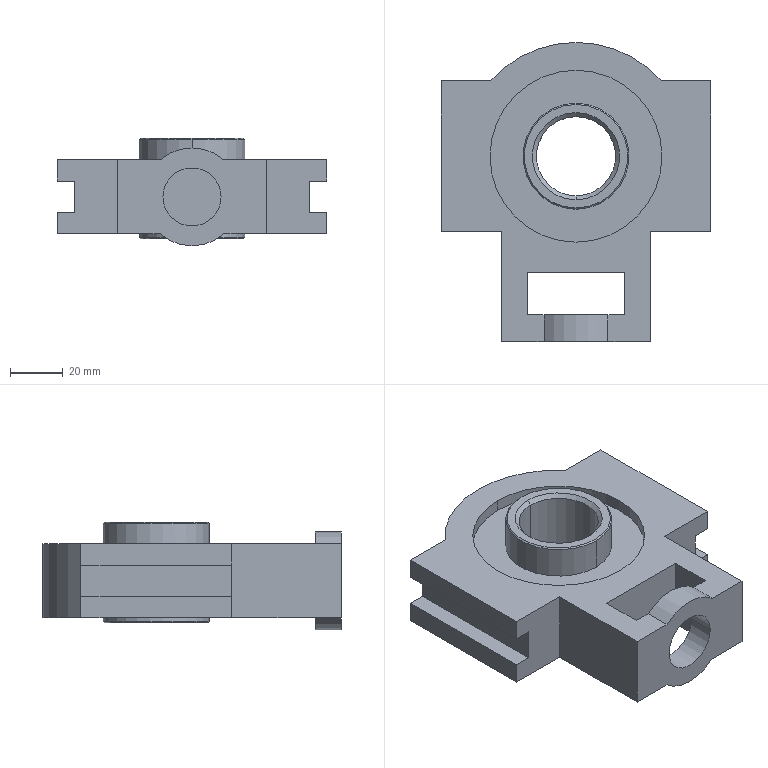Part | STEP file | uct206_011V11 | 1 solid | 50 faces | box 102 x 113 x 40.7 mm | volume 185287 mm3 | plane 27 | cylinder 15 | cone 8 | commonest cylinder face diameters 40.1 x4 65 x4 22 x2 30 x2 37 x2 86 x1